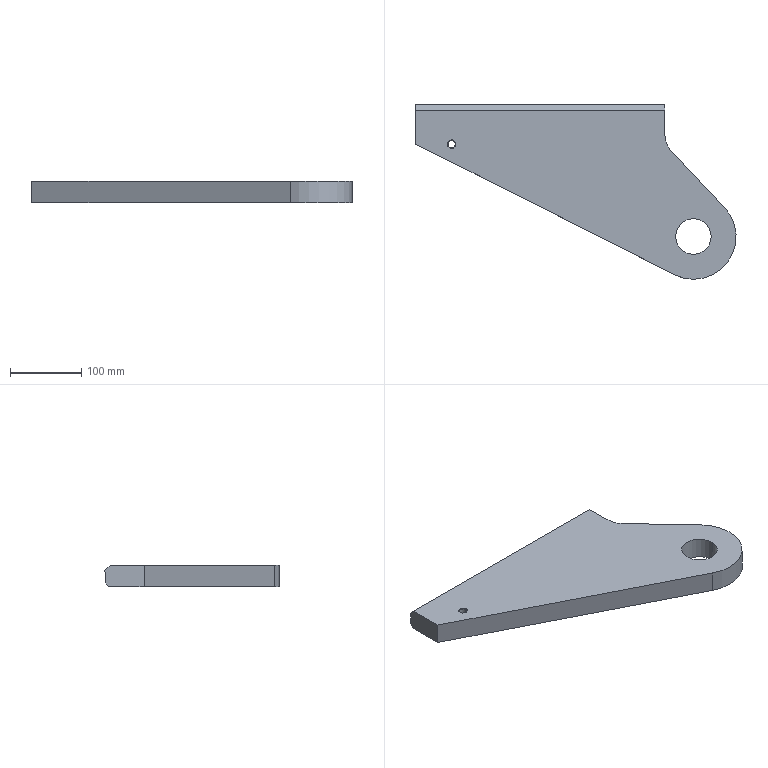Part | SolidWorks | features Chamfer 2, 3DProfileFeature 1, Extrusion 1, Fillet 1, HoleWzd 1, ICE 1 | 1 solid | 17 faces | box 450 x 245.418 x 30 mm | volume 1807994 mm3 | plane 8 | cylinder 7 | cone 2 | commonest cylinder face diameters 10.2 x2 50 x2 60 x1 110 x1 120 x1
STEP:
#1=CARTESIAN_POINT('',(-345.1,130.,29.075));
#2=VERTEX_POINT('',#1);
#3=CARTESIAN_POINT('',(-334.9,130.,29.075));
#4=VERTEX_POINT('',#3);
#5=CARTESIAN_POINT('',(-340.,130.,29.075));
#6=DIRECTION('',(0.,0.,1.));
#7=DIRECTION('',(1.,0.,0.));
#8=AXIS2_PLACEMENT_3D('',#5,#6,#7);
#9=CIRCLE('',#8,5.1);
#10=EDGE_CURVE('',#2,#4,#9,.T.);
#11=ORIENTED_EDGE('',*,*,#10,.F.);
#12=CARTESIAN_POINT('',(-346.025,130.,30.));
#13=VERTEX_POINT('',#12);
#14=CARTESIAN_POINT('',(-346.025,130.,30.));
#15=DIRECTION('',(-0.7071,0.,0.7071));
#16=VECTOR('',#15,1000.);
#17=LINE('',#14,#16);
#18=EDGE_CURVE('',#2,#13,#17,.T.);
#19=ORIENTED_EDGE('',*,*,#18,.T.);
#20=CARTESIAN_POINT('',(-333.975,130.,30.));
#21=VERTEX_POINT('',#20);
#22=CARTESIAN_POINT('',(-340.,130.,30.));
#23=DIRECTION('',(0.,0.,1.));
#24=DIRECTION('',(1.,0.,0.));
#25=AXIS2_PLACEMENT_3D('',#22,#23,#24);
#26=CIRCLE('',#25,6.025);
#27=EDGE_CURVE('',#13,#21,#26,.T.);
#28=ORIENTED_EDGE('',*,*,#27,.T.);
#29=CARTESIAN_POINT('',(-333.975,130.,30.));
#30=DIRECTION('',(0.7071,0.,0.7071));
#31=VECTOR('',#30,1000.);
#32=LINE('',#29,#31);
#33=EDGE_CURVE('',#4,#21,#32,.T.);
#34=ORIENTED_EDGE('',*,*,#33,.F.);
#35=EDGE_LOOP('',(#11,#19,#28,#34));
#36=FACE_OUTER_BOUND('',#35,.T.);
#37=CARTESIAN_POINT('',(-340.,130.,30.));
#38=DIRECTION('',(0.,0.,1.));
#39=DIRECTION('',(1.,0.,0.));
#40=AXIS2_PLACEMENT_3D('',#37,#38,#39);
#41=CONICAL_SURFACE('',#40,6.025,0.7854);
#42=ADVANCED_FACE('',(#36),#41,.F.);
#43=CARTESIAN_POINT('',(-345.1,130.,0.));
#44=VERTEX_POINT('',#43);
#45=CARTESIAN_POINT('',(-334.9,130.,0.));
#46=VERTEX_POINT('',#45);
#47=CARTESIAN_POINT('',(-340.,130.,0.));
#48=DIRECTION('',(0.,0.,1.));
#49=DIRECTION('',(1.,0.,0.));
#50=AXIS2_PLACEMENT_3D('',#47,#48,#49);
#51=CIRCLE('',#50,5.1);
#52=EDGE_CURVE('',#44,#46,#51,.T.);
#53=ORIENTED_EDGE('',*,*,#52,.F.);
#54=CARTESIAN_POINT('',(-345.1,130.,30.));
#55=DIRECTION('',(0.,0.,1.));
#56=VECTOR('',#55,1000.);
#57=LINE('',#54,#56);
#58=EDGE_CURVE('',#44,#2,#57,.T.);
#59=ORIENTED_EDGE('',*,*,#58,.T.);
#60=ORIENTED_EDGE('',*,*,#10,.T.);
#61=CARTESIAN_POINT('',(-334.9,130.,30.));
#62=DIRECTION('',(0.,0.,1.));
#63=VECTOR('',#62,1000.);
#64=LINE('',#61,#63);
#65=EDGE_CURVE('',#46,#4,#64,.T.);
#66=ORIENTED_EDGE('',*,*,#65,.F.);
#67=EDGE_LOOP('',(#53,#59,#60,#66));
#68=FACE_OUTER_BOUND('',#67,.T.);
#69=CARTESIAN_POINT('',(-340.,130.,30.));
#70=DIRECTION('',(0.,0.,1.));
#71=DIRECTION('',(1.,0.,0.));
#72=AXIS2_PLACEMENT_3D('',#69,#70,#71);
#73=CYLINDRICAL_SURFACE('',#72,5.1);
#74=ADVANCED_FACE('',(#68),#73,.F.);
#75=CARTESIAN_POINT('',(-25.,0.,30.));
#76=VERTEX_POINT('',#75);
#77=CARTESIAN_POINT('',(25.,0.,30.));
#78=VERTEX_POINT('',#77);
#79=CARTESIAN_POINT('',(0.,0.,30.));
#80=DIRECTION('',(0.,0.,1.));
#81=DIRECTION('',(1.,0.,0.));
#82=AXIS2_PLACEMENT_3D('',#79,#80,#81);
#83=CIRCLE('',#82,25.);
#84=EDGE_CURVE('',#76,#78,#83,.T.);
#85=ORIENTED_EDGE('',*,*,#84,.T.);
#86=CARTESIAN_POINT('',(25.,0.,0.));
#87=VERTEX_POINT('',#86);
#88=CARTESIAN_POINT('',(25.,0.,30.));
#89=DIRECTION('',(0.,0.,-1.));
#90=VECTOR('',#89,1000.);
#91=LINE('',#88,#90);
#92=EDGE_CURVE('',#78,#87,#91,.T.);
#93=ORIENTED_EDGE('',*,*,#92,.T.);
#94=CARTESIAN_POINT('',(-25.,0.,0.));
#95=VERTEX_POINT('',#94);
#96=CARTESIAN_POINT('',(0.,0.,0.));
#97=DIRECTION('',(0.,0.,1.));
#98=DIRECTION('',(1.,0.,0.));
#99=AXIS2_PLACEMENT_3D('',#96,#97,#98);
#100=CIRCLE('',#99,25.);
#101=EDGE_CURVE('',#95,#87,#100,.T.);
#102=ORIENTED_EDGE('',*,*,#101,.F.);
#103=CARTESIAN_POINT('',(-25.,0.,30.));
#104=DIRECTION('',(0.,0.,-1.));
#105=VECTOR('',#104,1000.);
#106=LINE('',#103,#105);
#107=EDGE_CURVE('',#76,#95,#106,.T.);
#108=ORIENTED_EDGE('',*,*,#107,.F.);
#109=EDGE_LOOP('',(#85,#93,#102,#108));
#110=FACE_OUTER_BOUND('',#109,.T.);
#111=CARTESIAN_POINT('',(0.,0.,30.));
#112=DIRECTION('',(0.,0.,-1.));
#113=DIRECTION('',(-1.,0.,0.));
#114=AXIS2_PLACEMENT_3D('',#111,#112,#113);
#115=CYLINDRICAL_SURFACE('',#114,25.);
#116=ADVANCED_FACE('',(#110),#115,.F.);
#117=CARTESIAN_POINT('',(-340.,130.,30.));
#118=DIRECTION('',(0.,0.,1.));
#119=DIRECTION('',(1.,0.,0.));
#120=AXIS2_PLACEMENT_3D('',#117,#118,#119);
#121=CIRCLE('',#120,6.025);
#122=EDGE_CURVE('',#21,#13,#121,.T.);
#123=ORIENTED_EDGE('',*,*,#122,.F.);
#124=ORIENTED_EDGE('',*,*,#27,.F.);
#125=EDGE_LOOP('',(#123,#124));
#126=FACE_BOUND('',#125,.T.);
#127=CARTESIAN_POINT('',(43.682,41.133,30.));
#128=VERTEX_POINT('',#127);
#129=CARTESIAN_POINT('',(-31.841,121.335,30.));
#130=VERTEX_POINT('',#129);
#131=CARTESIAN_POINT('',(-40.,130.,30.));
#132=DIRECTION('',(-0.6855,0.728,0.));
#133=VECTOR('',#132,1000.);
#134=LINE('',#131,#133);
#135=EDGE_CURVE('',#128,#130,#134,.T.);
#136=ORIENTED_EDGE('',*,*,#135,.T.);
#137=CARTESIAN_POINT('',(-40.,141.902,30.));
#138=VERTEX_POINT('',#137);
#139=CARTESIAN_POINT('',(-10.,141.902,30.));
#140=DIRECTION('',(0.,0.,-1.));
#141=DIRECTION('',(1.,0.,0.));
#142=AXIS2_PLACEMENT_3D('',#139,#140,#141);
#143=CIRCLE('',#142,30.);
#144=EDGE_CURVE('',#130,#138,#143,.T.);
#145=ORIENTED_EDGE('',*,*,#144,.T.);
#146=CARTESIAN_POINT('',(-40.,177.805,30.));
#147=VERTEX_POINT('',#146);
#148=CARTESIAN_POINT('',(-40.,250.,30.));
#149=DIRECTION('',(0.,1.,0.));
#150=VECTOR('',#149,1000.);
#151=LINE('',#148,#150);
#152=EDGE_CURVE('',#138,#147,#151,.T.);
#153=ORIENTED_EDGE('',*,*,#152,.T.);
#154=CARTESIAN_POINT('',(-390.,177.805,30.));
#155=VERTEX_POINT('',#154);
#156=CARTESIAN_POINT('',(-390.,177.805,30.));
#157=DIRECTION('',(-1.,0.,0.));
#158=VECTOR('',#157,1000.);
#159=LINE('',#156,#158);
#160=EDGE_CURVE('',#147,#155,#159,.T.);
#161=ORIENTED_EDGE('',*,*,#160,.T.);
#162=CARTESIAN_POINT('',(-390.,130.,30.));
#163=VERTEX_POINT('',#162);
#164=CARTESIAN_POINT('',(-390.,250.,30.));
#165=DIRECTION('',(0.,-1.,0.));
#166=VECTOR('',#165,1000.);
#167=LINE('',#164,#166);
#168=EDGE_CURVE('',#155,#163,#167,.T.);
#169=ORIENTED_EDGE('',*,*,#168,.T.);
#170=CARTESIAN_POINT('',(-27.078,-53.542,30.));
#171=VERTEX_POINT('',#170);
#172=CARTESIAN_POINT('',(-390.,130.,30.));
#173=DIRECTION('',(0.8924,-0.4513,0.));
#174=VECTOR('',#173,1000.);
#175=LINE('',#172,#174);
#176=EDGE_CURVE('',#163,#171,#175,.T.);
#177=ORIENTED_EDGE('',*,*,#176,.T.);
#178=CARTESIAN_POINT('',(0.,0.,30.));
#179=DIRECTION('',(0.,0.,1.));
#180=DIRECTION('',(1.,0.,0.));
#181=AXIS2_PLACEMENT_3D('',#178,#179,#180);
#182=CIRCLE('',#181,60.);
#183=EDGE_CURVE('',#171,#128,#182,.T.);
#184=ORIENTED_EDGE('',*,*,#183,.T.);
#185=EDGE_LOOP('',(#136,#145,#153,#161,#169,#177,#184));
#186=FACE_OUTER_BOUND('',#185,.T.);
#187=ORIENTED_EDGE('',*,*,#84,.F.);
#188=CARTESIAN_POINT('',(0.,0.,30.));
#189=DIRECTION('',(0.,0.,1.));
#190=DIRECTION('',(1.,0.,0.));
#191=AXIS2_PLACEMENT_3D('',#188,#189,#190);
#192=CIRCLE('',#191,25.);
#193=EDGE_CURVE('',#78,#76,#192,.T.);
#194=ORIENTED_EDGE('',*,*,#193,.F.);
#195=EDGE_LOOP('',(#187,#194));
#196=FACE_BOUND('',#195,.T.);
#197=CARTESIAN_POINT('',(0.,0.,30.));
#198=DIRECTION('',(0.,0.,1.));
#199=DIRECTION('',(1.,0.,0.));
#200=AXIS2_PLACEMENT_3D('',#197,#198,#199);
#201=PLANE('',#200);
#202=ADVANCED_FACE('',(#126,#186,#196),#201,.T.);
#203=CARTESIAN_POINT('',(-340.,130.,0.));
#204=DIRECTION('',(0.,0.,1.));
#205=DIRECTION('',(1.,0.,0.));
#206=AXIS2_PLACEMENT_3D('',#203,#204,#205);
#207=CIRCLE('',#206,5.1);
#208=EDGE_CURVE('',#46,#44,#207,.T.);
#209=ORIENTED_EDGE('',*,*,#208,.T.);
#210=ORIENTED_EDGE('',*,*,#52,.T.);
#211=EDGE_LOOP('',(#209,#210));
#212=FACE_BOUND('',#211,.T.);
#213=CARTESIAN_POINT('',(-390.,180.528,0.));
#214=VERTEX_POINT('',#213);
#215=CARTESIAN_POINT('',(-390.,130.,0.));
#216=VERTEX_POINT('',#215);
#217=CARTESIAN_POINT('',(-390.,250.,0.));
#218=DIRECTION('',(0.,-1.,0.));
#219=VECTOR('',#218,1000.);
#220=LINE('',#217,#219);
#221=EDGE_CURVE('',#214,#216,#220,.T.);
#222=ORIENTED_EDGE('',*,*,#221,.F.);
#223=CARTESIAN_POINT('',(-40.,180.528,0.));
#224=VERTEX_POINT('',#223);
#225=CARTESIAN_POINT('',(0.,180.528,0.));
#226=DIRECTION('',(1.,0.,0.));
#227=VECTOR('',#226,1000.);
#228=LINE('',#225,#227);
#229=EDGE_CURVE('',#214,#224,#228,.T.);
#230=ORIENTED_EDGE('',*,*,#229,.T.);
#231=CARTESIAN_POINT('',(-40.,141.902,0.));
#232=VERTEX_POINT('',#231);
#233=CARTESIAN_POINT('',(-40.,250.,0.));
#234=DIRECTION('',(0.,1.,0.));
#235=VECTOR('',#234,1000.);
#236=LINE('',#233,#235);
#237=EDGE_CURVE('',#232,#224,#236,.T.);
#238=ORIENTED_EDGE('',*,*,#237,.F.);
#239=CARTESIAN_POINT('',(-31.841,121.335,0.));
#240=VERTEX_POINT('',#239);
#241=CARTESIAN_POINT('',(-10.,141.902,0.));
#242=DIRECTION('',(0.,0.,1.));
#243=DIRECTION('',(1.,0.,0.));
#244=AXIS2_PLACEMENT_3D('',#241,#242,#243);
#245=CIRCLE('',#244,30.);
#246=EDGE_CURVE('',#232,#240,#245,.T.);
#247=ORIENTED_EDGE('',*,*,#246,.T.);
#248=CARTESIAN_POINT('',(43.682,41.133,0.));
#249=VERTEX_POINT('',#248);
#250=CARTESIAN_POINT('',(-40.,130.,0.));
#251=DIRECTION('',(-0.6855,0.728,0.));
#252=VECTOR('',#251,1000.);
#253=LINE('',#250,#252);
#254=EDGE_CURVE('',#249,#240,#253,.T.);
#255=ORIENTED_EDGE('',*,*,#254,.F.);
#256=CARTESIAN_POINT('',(-27.078,-53.542,0.));
#257=VERTEX_POINT('',#256);
#258=CARTESIAN_POINT('',(0.,0.,0.));
#259=DIRECTION('',(0.,0.,1.));
#260=DIRECTION('',(1.,0.,0.));
#261=AXIS2_PLACEMENT_3D('',#258,#259,#260);
#262=CIRCLE('',#261,60.);
#263=EDGE_CURVE('',#257,#249,#262,.T.);
#264=ORIENTED_EDGE('',*,*,#263,.F.);
#265=CARTESIAN_POINT('',(-390.,130.,0.));
#266=DIRECTION('',(0.8924,-0.4513,0.));
#267=VECTOR('',#266,1000.);
#268=LINE('',#265,#267);
#269=EDGE_CURVE('',#216,#257,#268,.T.);
#270=ORIENTED_EDGE('',*,*,#269,.F.);
#271=EDGE_LOOP('',(#222,#230,#238,#247,#255,#264,#270));
#272=FACE_OUTER_BOUND('',#271,.T.);
#273=ORIENTED_EDGE('',*,*,#101,.T.);
#274=CARTESIAN_POINT('',(0.,0.,0.));
#275=DIRECTION('',(0.,0.,1.));
#276=DIRECTION('',(1.,0.,0.));
#277=AXIS2_PLACEMENT_3D('',#274,#275,#276);
#278=CIRCLE('',#277,25.);
#279=EDGE_CURVE('',#87,#95,#278,.T.);
#280=ORIENTED_EDGE('',*,*,#279,.T.);
#281=EDGE_LOOP('',(#273,#280));
#282=FACE_BOUND('',#281,.T.);
#283=CARTESIAN_POINT('',(0.,0.,0.));
#284=DIRECTION('',(0.,0.,1.));
#285=DIRECTION('',(1.,0.,0.));
#286=AXIS2_PLACEMENT_3D('',#283,#284,#285);
#287=PLANE('',#286);
#288=ADVANCED_FACE('',(#212,#272,#282),#287,.F.);
#289=ORIENTED_EDGE('',*,*,#152,.F.);
#290=CARTESIAN_POINT('',(-40.,141.902,0.));
#291=DIRECTION('',(0.,0.,-1.));
#292=VECTOR('',#291,1000.);
#293=LINE('',#290,#292);
#294=EDGE_CURVE('',#138,#232,#293,.T.);
#295=ORIENTED_EDGE('',*,*,#294,.T.);
#296=ORIENTED_EDGE('',*,*,#237,.T.);
#297=CARTESIAN_POINT('',(-40.,184.145,5.212));
#298=VERTEX_POINT('',#297);
#299=CARTESIAN_POINT('',(-40.,180.528,0.));
#300=DIRECTION('',(0.,0.5701,0.8216));
#301=VECTOR('',#300,1000.);
#302=LINE('',#299,#301);
#303=EDGE_CURVE('',#224,#298,#302,.T.);
#304=ORIENTED_EDGE('',*,*,#303,.T.);
#305=CARTESIAN_POINT('',(-40.,185.418,22.387));
#306=VERTEX_POINT('',#305);
#307=CARTESIAN_POINT('',(-40.,238.954,9.782));
#308=DIRECTION('',(-1.,0.,0.));
#309=DIRECTION('',(0.,0.,1.));
#310=AXIS2_PLACEMENT_3D('',#307,#308,#309);
#311=CIRCLE('',#310,55.);
#312=EDGE_CURVE('',#298,#306,#311,.T.);
#313=ORIENTED_EDGE('',*,*,#312,.T.);
#314=CARTESIAN_POINT('',(-40.,185.418,22.387));
#315=DIRECTION('',(0.,-0.7071,0.7071));
#316=VECTOR('',#315,1000.);
#317=LINE('',#314,#316);
#318=EDGE_CURVE('',#306,#147,#317,.T.);
#319=ORIENTED_EDGE('',*,*,#318,.T.);
#320=EDGE_LOOP('',(#289,#295,#296,#304,#313,#319));
#321=FACE_OUTER_BOUND('',#320,.T.);
#322=CARTESIAN_POINT('',(-40.,250.,30.));
#323=DIRECTION('',(-1.,0.,0.));
#324=DIRECTION('',(0.,0.,1.));
#325=AXIS2_PLACEMENT_3D('',#322,#323,#324);
#326=PLANE('',#325);
#327=ADVANCED_FACE('',(#321),#326,.F.);
#328=CARTESIAN_POINT('',(-390.,185.418,22.387));
#329=VERTEX_POINT('',#328);
#330=CARTESIAN_POINT('',(-390.,184.145,5.212));
#331=VERTEX_POINT('',#330);
#332=CARTESIAN_POINT('',(-390.,238.954,9.782));
#333=DIRECTION('',(1.,0.,0.));
#334=DIRECTION('',(0.,1.,0.));
#335=AXIS2_PLACEMENT_3D('',#332,#333,#334);
#336=CIRCLE('',#335,55.);
#337=EDGE_CURVE('',#329,#331,#336,.T.);
#338=ORIENTED_EDGE('',*,*,#337,.T.);
#339=CARTESIAN_POINT('',(-390.,180.528,0.));
#340=DIRECTION('',(0.,-0.5701,-0.8216));
#341=VECTOR('',#340,1000.);
#342=LINE('',#339,#341);
#343=EDGE_CURVE('',#331,#214,#342,.T.);
#344=ORIENTED_EDGE('',*,*,#343,.T.);
#345=ORIENTED_EDGE('',*,*,#221,.T.);
#346=CARTESIAN_POINT('',(-390.,130.,30.));
#347=DIRECTION('',(0.,0.,-1.));
#348=VECTOR('',#347,1000.);
#349=LINE('',#346,#348);
#350=EDGE_CURVE('',#163,#216,#349,.T.);
#351=ORIENTED_EDGE('',*,*,#350,.F.);
#352=ORIENTED_EDGE('',*,*,#168,.F.);
#353=CARTESIAN_POINT('',(-390.,185.418,22.387));
#354=DIRECTION('',(0.,0.7071,-0.7071));
#355=VECTOR('',#354,1000.);
#356=LINE('',#353,#355);
#357=EDGE_CURVE('',#155,#329,#356,.T.);
#358=ORIENTED_EDGE('',*,*,#357,.T.);
#359=EDGE_LOOP('',(#338,#344,#345,#351,#352,#358));
#360=FACE_OUTER_BOUND('',#359,.T.);
#361=CARTESIAN_POINT('',(-390.,250.,30.));
#362=DIRECTION('',(1.,0.,0.));
#363=DIRECTION('',(0.,1.,0.));
#364=AXIS2_PLACEMENT_3D('',#361,#362,#363);
#365=PLANE('',#364);
#366=ADVANCED_FACE('',(#360),#365,.F.);
#367=ORIENTED_EDGE('',*,*,#269,.T.);
#368=CARTESIAN_POINT('',(-27.078,-53.542,30.));
#369=DIRECTION('',(0.,0.,-1.));
#370=VECTOR('',#369,1000.);
#371=LINE('',#368,#370);
#372=EDGE_CURVE('',#171,#257,#371,.T.);
#373=ORIENTED_EDGE('',*,*,#372,.F.);
#374=ORIENTED_EDGE('',*,*,#176,.F.);
#375=ORIENTED_EDGE('',*,*,#350,.T.);
#376=EDGE_LOOP('',(#367,#373,#374,#375));
#377=FACE_OUTER_BOUND('',#376,.T.);
#378=CARTESIAN_POINT('',(-390.,130.,30.));
#379=DIRECTION('',(0.4513,0.8924,0.));
#380=DIRECTION('',(-0.8924,0.4513,0.));
#381=AXIS2_PLACEMENT_3D('',#378,#379,#380);
#382=PLANE('',#381);
#383=ADVANCED_FACE('',(#377),#382,.F.);
#384=ORIENTED_EDGE('',*,*,#263,.T.);
#385=CARTESIAN_POINT('',(43.682,41.133,30.));
#386=DIRECTION('',(0.,0.,-1.));
#387=VECTOR('',#386,1000.);
#388=LINE('',#385,#387);
#389=EDGE_CURVE('',#128,#249,#388,.T.);
#390=ORIENTED_EDGE('',*,*,#389,.F.);
#391=ORIENTED_EDGE('',*,*,#183,.F.);
#392=ORIENTED_EDGE('',*,*,#372,.T.);
#393=EDGE_LOOP('',(#384,#390,#391,#392));
#394=FACE_OUTER_BOUND('',#393,.T.);
#395=CARTESIAN_POINT('',(0.,0.,30.));
#396=DIRECTION('',(0.,0.,-1.));
#397=DIRECTION('',(-1.,0.,0.));
#398=AXIS2_PLACEMENT_3D('',#395,#396,#397);
#399=CYLINDRICAL_SURFACE('',#398,60.);
#400=ADVANCED_FACE('',(#394),#399,.T.);
#401=ORIENTED_EDGE('',*,*,#254,.T.);
#402=CARTESIAN_POINT('',(-31.841,121.335,30.));
#403=DIRECTION('',(0.,0.,1.));
#404=VECTOR('',#403,1000.);
#405=LINE('',#402,#404);
#406=EDGE_CURVE('',#240,#130,#405,.T.);
#407=ORIENTED_EDGE('',*,*,#406,.T.);
#408=ORIENTED_EDGE('',*,*,#135,.F.);
#409=ORIENTED_EDGE('',*,*,#389,.T.);
#410=EDGE_LOOP('',(#401,#407,#408,#409));
#411=FACE_OUTER_BOUND('',#410,.T.);
#412=CARTESIAN_POINT('',(-40.,130.,30.));
#413=DIRECTION('',(-0.728,-0.6855,0.));
#414=DIRECTION('',(0.6855,-0.728,0.));
#415=AXIS2_PLACEMENT_3D('',#412,#413,#414);
#416=PLANE('',#415);
#417=ADVANCED_FACE('',(#411),#416,.F.);
#418=ORIENTED_EDGE('',*,*,#92,.F.);
#419=ORIENTED_EDGE('',*,*,#193,.T.);
#420=ORIENTED_EDGE('',*,*,#107,.T.);
#421=ORIENTED_EDGE('',*,*,#279,.F.);
#422=EDGE_LOOP('',(#418,#419,#420,#421));
#423=FACE_OUTER_BOUND('',#422,.T.);
#424=CARTESIAN_POINT('',(0.,0.,30.));
#425=DIRECTION('',(0.,0.,-1.));
#426=DIRECTION('',(-1.,0.,0.));
#427=AXIS2_PLACEMENT_3D('',#424,#425,#426);
#428=CYLINDRICAL_SURFACE('',#427,25.);
#429=ADVANCED_FACE('',(#423),#428,.F.);
#430=ORIENTED_EDGE('',*,*,#312,.F.);
#431=CARTESIAN_POINT('',(-390.,184.145,5.212));
#432=DIRECTION('',(-1.,0.,0.));
#433=VECTOR('',#432,1000.);
#434=LINE('',#431,#433);
#435=EDGE_CURVE('',#298,#331,#434,.T.);
#436=ORIENTED_EDGE('',*,*,#435,.T.);
#437=ORIENTED_EDGE('',*,*,#337,.F.);
#438=CARTESIAN_POINT('',(-390.,185.418,22.387));
#439=DIRECTION('',(1.,0.,0.));
#440=VECTOR('',#439,1000.);
#441=LINE('',#438,#440);
#442=EDGE_CURVE('',#329,#306,#441,.T.);
#443=ORIENTED_EDGE('',*,*,#442,.T.);
#444=EDGE_LOOP('',(#430,#436,#437,#443));
#445=FACE_OUTER_BOUND('',#444,.T.);
#446=CARTESIAN_POINT('',(-390.,238.954,9.782));
#447=DIRECTION('',(1.,0.,0.));
#448=DIRECTION('',(0.,1.,0.));
#449=AXIS2_PLACEMENT_3D('',#446,#447,#448);
#450=CYLINDRICAL_SURFACE('',#449,55.);
#451=ADVANCED_FACE('',(#445),#450,.F.);
#452=ORIENTED_EDGE('',*,*,#357,.F.);
#453=ORIENTED_EDGE('',*,*,#160,.F.);
#454=ORIENTED_EDGE('',*,*,#318,.F.);
#455=ORIENTED_EDGE('',*,*,#442,.F.);
#456=EDGE_LOOP('',(#452,#453,#454,#455));
#457=FACE_OUTER_BOUND('',#456,.T.);
#458=CARTESIAN_POINT('',(-390.,185.418,22.387));
#459=DIRECTION('',(0.,-0.7071,-0.7071));
#460=DIRECTION('',(1.,0.,0.));
#461=AXIS2_PLACEMENT_3D('',#458,#459,#460);
#462=PLANE('',#461);
#463=ADVANCED_FACE('',(#457),#462,.F.);
#464=ORIENTED_EDGE('',*,*,#343,.F.);
#465=ORIENTED_EDGE('',*,*,#435,.F.);
#466=ORIENTED_EDGE('',*,*,#303,.F.);
#467=ORIENTED_EDGE('',*,*,#229,.F.);
#468=EDGE_LOOP('',(#464,#465,#466,#467));
#469=FACE_OUTER_BOUND('',#468,.T.);
#470=CARTESIAN_POINT('',(-390.,180.528,0.));
#471=DIRECTION('',(0.,-0.8216,0.5701));
#472=DIRECTION('',(1.,0.,0.));
#473=AXIS2_PLACEMENT_3D('',#470,#471,#472);
#474=PLANE('',#473);
#475=ADVANCED_FACE('',(#469),#474,.F.);
#476=ORIENTED_EDGE('',*,*,#144,.F.);
#477=ORIENTED_EDGE('',*,*,#406,.F.);
#478=ORIENTED_EDGE('',*,*,#246,.F.);
#479=ORIENTED_EDGE('',*,*,#294,.F.);
#480=EDGE_LOOP('',(#476,#477,#478,#479));
#481=FACE_OUTER_BOUND('',#480,.T.);
#482=CARTESIAN_POINT('',(-10.,141.902,30.));
#483=DIRECTION('',(0.,0.,1.));
#484=DIRECTION('',(1.,0.,0.));
#485=AXIS2_PLACEMENT_3D('',#482,#483,#484);
#486=CYLINDRICAL_SURFACE('',#485,30.);
#487=ADVANCED_FACE('',(#481),#486,.F.);
#488=ORIENTED_EDGE('',*,*,#58,.F.);
#489=ORIENTED_EDGE('',*,*,#208,.F.);
#490=ORIENTED_EDGE('',*,*,#65,.T.);
#491=CARTESIAN_POINT('',(-340.,130.,29.075));
#492=DIRECTION('',(0.,0.,1.));
#493=DIRECTION('',(1.,0.,0.));
#494=AXIS2_PLACEMENT_3D('',#491,#492,#493);
#495=CIRCLE('',#494,5.1);
#496=EDGE_CURVE('',#4,#2,#495,.T.);
#497=ORIENTED_EDGE('',*,*,#496,.T.);
#498=EDGE_LOOP('',(#488,#489,#490,#497));
#499=FACE_OUTER_BOUND('',#498,.T.);
#500=CARTESIAN_POINT('',(-340.,130.,30.));
#501=DIRECTION('',(0.,0.,1.));
#502=DIRECTION('',(1.,0.,0.));
#503=AXIS2_PLACEMENT_3D('',#500,#501,#502);
#504=CYLINDRICAL_SURFACE('',#503,5.1);
#505=ADVANCED_FACE('',(#499),#504,.F.);
#506=ORIENTED_EDGE('',*,*,#18,.F.);
#507=ORIENTED_EDGE('',*,*,#496,.F.);
#508=ORIENTED_EDGE('',*,*,#33,.T.);
#509=ORIENTED_EDGE('',*,*,#122,.T.);
#510=EDGE_LOOP('',(#506,#507,#508,#509));
#511=FACE_OUTER_BOUND('',#510,.T.);
#512=CARTESIAN_POINT('',(-340.,130.,30.));
#513=DIRECTION('',(0.,0.,1.));
#514=DIRECTION('',(1.,0.,0.));
#515=AXIS2_PLACEMENT_3D('',#512,#513,#514);
#516=CONICAL_SURFACE('',#515,6.025,0.7854);
#517=ADVANCED_FACE('',(#511),#516,.F.);
#518=CLOSED_SHELL('',(#42,#74,#116,#202,#288,#327,#366,#383,#400,#417,#429,#451,#463,#475,#487,#505,#517));
#519=MANIFOLD_SOLID_BREP('',#518);
#520=CARTESIAN_POINT('',(0.,0.,0.));
#521=DIRECTION('',(0.,0.,1.));
#522=DIRECTION('',(1.,0.,0.));
#523=AXIS2_PLACEMENT_3D('',#520,#521,#522);
#524=(LENGTH_UNIT()NAMED_UNIT(*)SI_UNIT(.MILLI.,.METRE.));
#525=UNCERTAINTY_MEASURE_WITH_UNIT(LENGTH_MEASURE(0.00001),#524,'','');
#526=(NAMED_UNIT(*)PLANE_ANGLE_UNIT()SI_UNIT($,.RADIAN.));
#527=(NAMED_UNIT(*)SI_UNIT($,.STERADIAN.)SOLID_ANGLE_UNIT());
#528=(GEOMETRIC_REPRESENTATION_CONTEXT(3)GLOBAL_UNCERTAINTY_ASSIGNED_CONTEXT((#525))GLOBAL_UNIT_ASSIGNED_CONTEXT((#524,#526,#527))REPRESENTATION_CONTEXT('',''));
#529=ADVANCED_BREP_SHAPE_REPRESENTATION('',(#519,#523),#528);